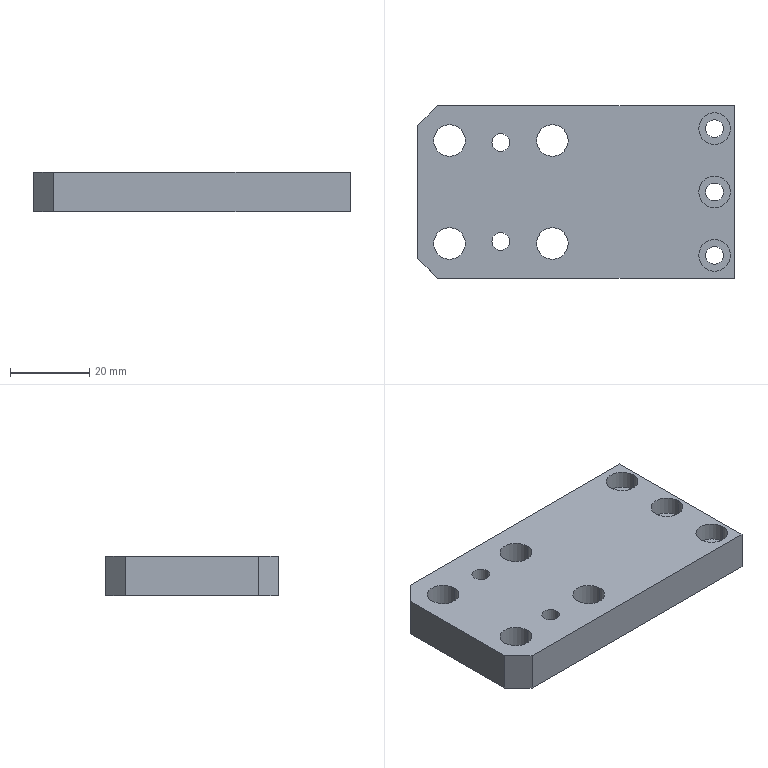Part | SolidWorks | features HoleWzd 3, Chamfer 1, Extrusion 1 | 1 solid | 41 faces | box 80 x 43.6 x 10 mm | volume 31034 mm3 | cylinder 28 | plane 13 | commonest cylinder face diameters 8 x18 4.5 x10
STEP:
#1=CARTESIAN_POINT('',(71.,37.8,-4.6));
#2=VERTEX_POINT('',#1);
#3=CARTESIAN_POINT('',(79.,37.8,-4.6));
#4=VERTEX_POINT('',#3);
#5=CARTESIAN_POINT('',(75.,37.8,-4.6));
#6=DIRECTION('',(0.,0.,1.));
#7=DIRECTION('',(1.,0.,0.));
#8=AXIS2_PLACEMENT_3D('',#5,#6,#7);
#9=CIRCLE('',#8,4.);
#10=EDGE_CURVE('',#2,#4,#9,.T.);
#11=ORIENTED_EDGE('',*,*,#10,.F.);
#12=CARTESIAN_POINT('',(71.,37.8,0.));
#13=VERTEX_POINT('',#12);
#14=CARTESIAN_POINT('',(71.,37.8,0.));
#15=DIRECTION('',(0.,0.,1.));
#16=VECTOR('',#15,1000.);
#17=LINE('',#14,#16);
#18=EDGE_CURVE('',#2,#13,#17,.T.);
#19=ORIENTED_EDGE('',*,*,#18,.T.);
#20=CARTESIAN_POINT('',(79.,37.8,0.));
#21=VERTEX_POINT('',#20);
#22=CARTESIAN_POINT('',(75.,37.8,0.));
#23=DIRECTION('',(0.,0.,1.));
#24=DIRECTION('',(1.,0.,0.));
#25=AXIS2_PLACEMENT_3D('',#22,#23,#24);
#26=CIRCLE('',#25,4.);
#27=EDGE_CURVE('',#13,#21,#26,.T.);
#28=ORIENTED_EDGE('',*,*,#27,.T.);
#29=CARTESIAN_POINT('',(79.,37.8,0.));
#30=DIRECTION('',(0.,0.,1.));
#31=VECTOR('',#30,1000.);
#32=LINE('',#29,#31);
#33=EDGE_CURVE('',#4,#21,#32,.T.);
#34=ORIENTED_EDGE('',*,*,#33,.F.);
#35=EDGE_LOOP('',(#11,#19,#28,#34));
#36=FACE_OUTER_BOUND('',#35,.T.);
#37=CARTESIAN_POINT('',(75.,37.8,0.));
#38=DIRECTION('',(0.,0.,1.));
#39=DIRECTION('',(1.,0.,0.));
#40=AXIS2_PLACEMENT_3D('',#37,#38,#39);
#41=CYLINDRICAL_SURFACE('',#40,4.);
#42=ADVANCED_FACE('',(#36),#41,.F.);
#43=CARTESIAN_POINT('',(72.75,37.8,-10.));
#44=VERTEX_POINT('',#43);
#45=CARTESIAN_POINT('',(77.25,37.8,-10.));
#46=VERTEX_POINT('',#45);
#47=CARTESIAN_POINT('',(75.,37.8,-10.));
#48=DIRECTION('',(0.,0.,1.));
#49=DIRECTION('',(1.,0.,0.));
#50=AXIS2_PLACEMENT_3D('',#47,#48,#49);
#51=CIRCLE('',#50,2.25);
#52=EDGE_CURVE('',#44,#46,#51,.T.);
#53=ORIENTED_EDGE('',*,*,#52,.F.);
#54=CARTESIAN_POINT('',(72.75,37.8,-4.6));
#55=VERTEX_POINT('',#54);
#56=CARTESIAN_POINT('',(72.75,37.8,0.));
#57=DIRECTION('',(0.,0.,1.));
#58=VECTOR('',#57,1000.);
#59=LINE('',#56,#58);
#60=EDGE_CURVE('',#44,#55,#59,.T.);
#61=ORIENTED_EDGE('',*,*,#60,.T.);
#62=CARTESIAN_POINT('',(77.25,37.8,-4.6));
#63=VERTEX_POINT('',#62);
#64=CARTESIAN_POINT('',(75.,37.8,-4.6));
#65=DIRECTION('',(0.,0.,1.));
#66=DIRECTION('',(1.,0.,0.));
#67=AXIS2_PLACEMENT_3D('',#64,#65,#66);
#68=CIRCLE('',#67,2.25);
#69=EDGE_CURVE('',#55,#63,#68,.T.);
#70=ORIENTED_EDGE('',*,*,#69,.T.);
#71=CARTESIAN_POINT('',(77.25,37.8,0.));
#72=DIRECTION('',(0.,0.,1.));
#73=VECTOR('',#72,1000.);
#74=LINE('',#71,#73);
#75=EDGE_CURVE('',#46,#63,#74,.T.);
#76=ORIENTED_EDGE('',*,*,#75,.F.);
#77=EDGE_LOOP('',(#53,#61,#70,#76));
#78=FACE_OUTER_BOUND('',#77,.T.);
#79=CARTESIAN_POINT('',(75.,37.8,0.));
#80=DIRECTION('',(0.,0.,1.));
#81=DIRECTION('',(1.,0.,0.));
#82=AXIS2_PLACEMENT_3D('',#79,#80,#81);
#83=CYLINDRICAL_SURFACE('',#82,2.25);
#84=ADVANCED_FACE('',(#78),#83,.F.);
#85=CARTESIAN_POINT('',(71.,5.8,-4.6));
#86=VERTEX_POINT('',#85);
#87=CARTESIAN_POINT('',(79.,5.8,-4.6));
#88=VERTEX_POINT('',#87);
#89=CARTESIAN_POINT('',(75.,5.8,-4.6));
#90=DIRECTION('',(0.,0.,1.));
#91=DIRECTION('',(1.,0.,0.));
#92=AXIS2_PLACEMENT_3D('',#89,#90,#91);
#93=CIRCLE('',#92,4.);
#94=EDGE_CURVE('',#86,#88,#93,.T.);
#95=ORIENTED_EDGE('',*,*,#94,.F.);
#96=CARTESIAN_POINT('',(71.,5.8,0.));
#97=VERTEX_POINT('',#96);
#98=CARTESIAN_POINT('',(71.,5.8,0.));
#99=DIRECTION('',(0.,0.,1.));
#100=VECTOR('',#99,1000.);
#101=LINE('',#98,#100);
#102=EDGE_CURVE('',#86,#97,#101,.T.);
#103=ORIENTED_EDGE('',*,*,#102,.T.);
#104=CARTESIAN_POINT('',(79.,5.8,0.));
#105=VERTEX_POINT('',#104);
#106=CARTESIAN_POINT('',(75.,5.8,0.));
#107=DIRECTION('',(0.,0.,1.));
#108=DIRECTION('',(1.,0.,0.));
#109=AXIS2_PLACEMENT_3D('',#106,#107,#108);
#110=CIRCLE('',#109,4.);
#111=EDGE_CURVE('',#97,#105,#110,.T.);
#112=ORIENTED_EDGE('',*,*,#111,.T.);
#113=CARTESIAN_POINT('',(79.,5.8,0.));
#114=DIRECTION('',(0.,0.,1.));
#115=VECTOR('',#114,1000.);
#116=LINE('',#113,#115);
#117=EDGE_CURVE('',#88,#105,#116,.T.);
#118=ORIENTED_EDGE('',*,*,#117,.F.);
#119=EDGE_LOOP('',(#95,#103,#112,#118));
#120=FACE_OUTER_BOUND('',#119,.T.);
#121=CARTESIAN_POINT('',(75.,5.8,0.));
#122=DIRECTION('',(0.,0.,1.));
#123=DIRECTION('',(1.,0.,0.));
#124=AXIS2_PLACEMENT_3D('',#121,#122,#123);
#125=CYLINDRICAL_SURFACE('',#124,4.);
#126=ADVANCED_FACE('',(#120),#125,.F.);
#127=CARTESIAN_POINT('',(72.75,5.8,-10.));
#128=VERTEX_POINT('',#127);
#129=CARTESIAN_POINT('',(77.25,5.8,-10.));
#130=VERTEX_POINT('',#129);
#131=CARTESIAN_POINT('',(75.,5.8,-10.));
#132=DIRECTION('',(0.,0.,1.));
#133=DIRECTION('',(1.,0.,0.));
#134=AXIS2_PLACEMENT_3D('',#131,#132,#133);
#135=CIRCLE('',#134,2.25);
#136=EDGE_CURVE('',#128,#130,#135,.T.);
#137=ORIENTED_EDGE('',*,*,#136,.F.);
#138=CARTESIAN_POINT('',(72.75,5.8,-4.6));
#139=VERTEX_POINT('',#138);
#140=CARTESIAN_POINT('',(72.75,5.8,0.));
#141=DIRECTION('',(0.,0.,1.));
#142=VECTOR('',#141,1000.);
#143=LINE('',#140,#142);
#144=EDGE_CURVE('',#128,#139,#143,.T.);
#145=ORIENTED_EDGE('',*,*,#144,.T.);
#146=CARTESIAN_POINT('',(77.25,5.8,-4.6));
#147=VERTEX_POINT('',#146);
#148=CARTESIAN_POINT('',(75.,5.8,-4.6));
#149=DIRECTION('',(0.,0.,1.));
#150=DIRECTION('',(1.,0.,0.));
#151=AXIS2_PLACEMENT_3D('',#148,#149,#150);
#152=CIRCLE('',#151,2.25);
#153=EDGE_CURVE('',#139,#147,#152,.T.);
#154=ORIENTED_EDGE('',*,*,#153,.T.);
#155=CARTESIAN_POINT('',(77.25,5.8,0.));
#156=DIRECTION('',(0.,0.,1.));
#157=VECTOR('',#156,1000.);
#158=LINE('',#155,#157);
#159=EDGE_CURVE('',#130,#147,#158,.T.);
#160=ORIENTED_EDGE('',*,*,#159,.F.);
#161=EDGE_LOOP('',(#137,#145,#154,#160));
#162=FACE_OUTER_BOUND('',#161,.T.);
#163=CARTESIAN_POINT('',(75.,5.8,0.));
#164=DIRECTION('',(0.,0.,1.));
#165=DIRECTION('',(1.,0.,0.));
#166=AXIS2_PLACEMENT_3D('',#163,#164,#165);
#167=CYLINDRICAL_SURFACE('',#166,2.25);
#168=ADVANCED_FACE('',(#162),#167,.F.);
#169=CARTESIAN_POINT('',(71.,21.8,-4.6));
#170=VERTEX_POINT('',#169);
#171=CARTESIAN_POINT('',(79.,21.8,-4.6));
#172=VERTEX_POINT('',#171);
#173=CARTESIAN_POINT('',(75.,21.8,-4.6));
#174=DIRECTION('',(0.,0.,1.));
#175=DIRECTION('',(1.,0.,0.));
#176=AXIS2_PLACEMENT_3D('',#173,#174,#175);
#177=CIRCLE('',#176,4.);
#178=EDGE_CURVE('',#170,#172,#177,.T.);
#179=ORIENTED_EDGE('',*,*,#178,.F.);
#180=CARTESIAN_POINT('',(71.,21.8,0.));
#181=VERTEX_POINT('',#180);
#182=CARTESIAN_POINT('',(71.,21.8,0.));
#183=DIRECTION('',(0.,0.,1.));
#184=VECTOR('',#183,1000.);
#185=LINE('',#182,#184);
#186=EDGE_CURVE('',#170,#181,#185,.T.);
#187=ORIENTED_EDGE('',*,*,#186,.T.);
#188=CARTESIAN_POINT('',(79.,21.8,0.));
#189=VERTEX_POINT('',#188);
#190=CARTESIAN_POINT('',(75.,21.8,0.));
#191=DIRECTION('',(0.,0.,1.));
#192=DIRECTION('',(1.,0.,0.));
#193=AXIS2_PLACEMENT_3D('',#190,#191,#192);
#194=CIRCLE('',#193,4.);
#195=EDGE_CURVE('',#181,#189,#194,.T.);
#196=ORIENTED_EDGE('',*,*,#195,.T.);
#197=CARTESIAN_POINT('',(79.,21.8,0.));
#198=DIRECTION('',(0.,0.,1.));
#199=VECTOR('',#198,1000.);
#200=LINE('',#197,#199);
#201=EDGE_CURVE('',#172,#189,#200,.T.);
#202=ORIENTED_EDGE('',*,*,#201,.F.);
#203=EDGE_LOOP('',(#179,#187,#196,#202));
#204=FACE_OUTER_BOUND('',#203,.T.);
#205=CARTESIAN_POINT('',(75.,21.8,0.));
#206=DIRECTION('',(0.,0.,1.));
#207=DIRECTION('',(1.,0.,0.));
#208=AXIS2_PLACEMENT_3D('',#205,#206,#207);
#209=CYLINDRICAL_SURFACE('',#208,4.);
#210=ADVANCED_FACE('',(#204),#209,.F.);
#211=CARTESIAN_POINT('',(72.75,21.8,-10.));
#212=VERTEX_POINT('',#211);
#213=CARTESIAN_POINT('',(77.25,21.8,-10.));
#214=VERTEX_POINT('',#213);
#215=CARTESIAN_POINT('',(75.,21.8,-10.));
#216=DIRECTION('',(0.,0.,1.));
#217=DIRECTION('',(1.,0.,0.));
#218=AXIS2_PLACEMENT_3D('',#215,#216,#217);
#219=CIRCLE('',#218,2.25);
#220=EDGE_CURVE('',#212,#214,#219,.T.);
#221=ORIENTED_EDGE('',*,*,#220,.F.);
#222=CARTESIAN_POINT('',(72.75,21.8,-4.6));
#223=VERTEX_POINT('',#222);
#224=CARTESIAN_POINT('',(72.75,21.8,0.));
#225=DIRECTION('',(0.,0.,1.));
#226=VECTOR('',#225,1000.);
#227=LINE('',#224,#226);
#228=EDGE_CURVE('',#212,#223,#227,.T.);
#229=ORIENTED_EDGE('',*,*,#228,.T.);
#230=CARTESIAN_POINT('',(77.25,21.8,-4.6));
#231=VERTEX_POINT('',#230);
#232=CARTESIAN_POINT('',(75.,21.8,-4.6));
#233=DIRECTION('',(0.,0.,1.));
#234=DIRECTION('',(1.,0.,0.));
#235=AXIS2_PLACEMENT_3D('',#232,#233,#234);
#236=CIRCLE('',#235,2.25);
#237=EDGE_CURVE('',#223,#231,#236,.T.);
#238=ORIENTED_EDGE('',*,*,#237,.T.);
#239=CARTESIAN_POINT('',(77.25,21.8,0.));
#240=DIRECTION('',(0.,0.,1.));
#241=VECTOR('',#240,1000.);
#242=LINE('',#239,#241);
#243=EDGE_CURVE('',#214,#231,#242,.T.);
#244=ORIENTED_EDGE('',*,*,#243,.F.);
#245=EDGE_LOOP('',(#221,#229,#238,#244));
#246=FACE_OUTER_BOUND('',#245,.T.);
#247=CARTESIAN_POINT('',(75.,21.8,0.));
#248=DIRECTION('',(0.,0.,1.));
#249=DIRECTION('',(1.,0.,0.));
#250=AXIS2_PLACEMENT_3D('',#247,#248,#249);
#251=CYLINDRICAL_SURFACE('',#250,2.25);
#252=ADVANCED_FACE('',(#246),#251,.F.);
#253=CARTESIAN_POINT('',(25.,34.3,-5.4));
#254=VERTEX_POINT('',#253);
#255=CARTESIAN_POINT('',(17.,34.3,-5.4));
#256=VERTEX_POINT('',#255);
#257=CARTESIAN_POINT('',(21.,34.3,-5.4));
#258=DIRECTION('',(0.,0.,-1.));
#259=DIRECTION('',(-1.,0.,0.));
#260=AXIS2_PLACEMENT_3D('',#257,#258,#259);
#261=CIRCLE('',#260,4.);
#262=EDGE_CURVE('',#254,#256,#261,.T.);
#263=ORIENTED_EDGE('',*,*,#262,.F.);
#264=CARTESIAN_POINT('',(25.,34.3,-10.));
#265=VERTEX_POINT('',#264);
#266=CARTESIAN_POINT('',(25.,34.3,-10.));
#267=DIRECTION('',(0.,0.,-1.));
#268=VECTOR('',#267,1000.);
#269=LINE('',#266,#268);
#270=EDGE_CURVE('',#254,#265,#269,.T.);
#271=ORIENTED_EDGE('',*,*,#270,.T.);
#272=CARTESIAN_POINT('',(17.,34.3,-10.));
#273=VERTEX_POINT('',#272);
#274=CARTESIAN_POINT('',(21.,34.3,-10.));
#275=DIRECTION('',(0.,0.,-1.));
#276=DIRECTION('',(-1.,0.,0.));
#277=AXIS2_PLACEMENT_3D('',#274,#275,#276);
#278=CIRCLE('',#277,4.);
#279=EDGE_CURVE('',#265,#273,#278,.T.);
#280=ORIENTED_EDGE('',*,*,#279,.T.);
#281=CARTESIAN_POINT('',(17.,34.3,-10.));
#282=DIRECTION('',(0.,0.,-1.));
#283=VECTOR('',#282,1000.);
#284=LINE('',#281,#283);
#285=EDGE_CURVE('',#256,#273,#284,.T.);
#286=ORIENTED_EDGE('',*,*,#285,.F.);
#287=EDGE_LOOP('',(#263,#271,#280,#286));
#288=FACE_OUTER_BOUND('',#287,.T.);
#289=CARTESIAN_POINT('',(21.,34.3,-10.));
#290=DIRECTION('',(0.,0.,-1.));
#291=DIRECTION('',(-1.,0.,0.));
#292=AXIS2_PLACEMENT_3D('',#289,#290,#291);
#293=CYLINDRICAL_SURFACE('',#292,4.);
#294=ADVANCED_FACE('',(#288),#293,.F.);
#295=CARTESIAN_POINT('',(23.25,34.3,0.));
#296=VERTEX_POINT('',#295);
#297=CARTESIAN_POINT('',(18.75,34.3,0.));
#298=VERTEX_POINT('',#297);
#299=CARTESIAN_POINT('',(21.,34.3,0.));
#300=DIRECTION('',(0.,0.,-1.));
#301=DIRECTION('',(-1.,0.,0.));
#302=AXIS2_PLACEMENT_3D('',#299,#300,#301);
#303=CIRCLE('',#302,2.25);
#304=EDGE_CURVE('',#296,#298,#303,.T.);
#305=ORIENTED_EDGE('',*,*,#304,.F.);
#306=CARTESIAN_POINT('',(23.25,34.3,-5.4));
#307=VERTEX_POINT('',#306);
#308=CARTESIAN_POINT('',(23.25,34.3,-10.));
#309=DIRECTION('',(0.,0.,-1.));
#310=VECTOR('',#309,1000.);
#311=LINE('',#308,#310);
#312=EDGE_CURVE('',#296,#307,#311,.T.);
#313=ORIENTED_EDGE('',*,*,#312,.T.);
#314=CARTESIAN_POINT('',(18.75,34.3,-5.4));
#315=VERTEX_POINT('',#314);
#316=CARTESIAN_POINT('',(21.,34.3,-5.4));
#317=DIRECTION('',(0.,0.,-1.));
#318=DIRECTION('',(-1.,0.,0.));
#319=AXIS2_PLACEMENT_3D('',#316,#317,#318);
#320=CIRCLE('',#319,2.25);
#321=EDGE_CURVE('',#307,#315,#320,.T.);
#322=ORIENTED_EDGE('',*,*,#321,.T.);
#323=CARTESIAN_POINT('',(18.75,34.3,-10.));
#324=DIRECTION('',(0.,0.,-1.));
#325=VECTOR('',#324,1000.);
#326=LINE('',#323,#325);
#327=EDGE_CURVE('',#298,#315,#326,.T.);
#328=ORIENTED_EDGE('',*,*,#327,.F.);
#329=EDGE_LOOP('',(#305,#313,#322,#328));
#330=FACE_OUTER_BOUND('',#329,.T.);
#331=CARTESIAN_POINT('',(21.,34.3,-10.));
#332=DIRECTION('',(0.,0.,-1.));
#333=DIRECTION('',(-1.,0.,0.));
#334=AXIS2_PLACEMENT_3D('',#331,#332,#333);
#335=CYLINDRICAL_SURFACE('',#334,2.25);
#336=ADVANCED_FACE('',(#330),#335,.F.);
#337=CARTESIAN_POINT('',(25.,9.3,-5.4));
#338=VERTEX_POINT('',#337);
#339=CARTESIAN_POINT('',(17.,9.3,-5.4));
#340=VERTEX_POINT('',#339);
#341=CARTESIAN_POINT('',(21.,9.3,-5.4));
#342=DIRECTION('',(0.,0.,-1.));
#343=DIRECTION('',(-1.,0.,0.));
#344=AXIS2_PLACEMENT_3D('',#341,#342,#343);
#345=CIRCLE('',#344,4.);
#346=EDGE_CURVE('',#338,#340,#345,.T.);
#347=ORIENTED_EDGE('',*,*,#346,.F.);
#348=CARTESIAN_POINT('',(25.,9.3,-10.));
#349=VERTEX_POINT('',#348);
#350=CARTESIAN_POINT('',(25.,9.3,-10.));
#351=DIRECTION('',(0.,0.,-1.));
#352=VECTOR('',#351,1000.);
#353=LINE('',#350,#352);
#354=EDGE_CURVE('',#338,#349,#353,.T.);
#355=ORIENTED_EDGE('',*,*,#354,.T.);
#356=CARTESIAN_POINT('',(17.,9.3,-10.));
#357=VERTEX_POINT('',#356);
#358=CARTESIAN_POINT('',(21.,9.3,-10.));
#359=DIRECTION('',(0.,0.,-1.));
#360=DIRECTION('',(-1.,0.,0.));
#361=AXIS2_PLACEMENT_3D('',#358,#359,#360);
#362=CIRCLE('',#361,4.);
#363=EDGE_CURVE('',#349,#357,#362,.T.);
#364=ORIENTED_EDGE('',*,*,#363,.T.);
#365=CARTESIAN_POINT('',(17.,9.3,-10.));
#366=DIRECTION('',(0.,0.,-1.));
#367=VECTOR('',#366,1000.);
#368=LINE('',#365,#367);
#369=EDGE_CURVE('',#340,#357,#368,.T.);
#370=ORIENTED_EDGE('',*,*,#369,.F.);
#371=EDGE_LOOP('',(#347,#355,#364,#370));
#372=FACE_OUTER_BOUND('',#371,.T.);
#373=CARTESIAN_POINT('',(21.,9.3,-10.));
#374=DIRECTION('',(0.,0.,-1.));
#375=DIRECTION('',(-1.,0.,0.));
#376=AXIS2_PLACEMENT_3D('',#373,#374,#375);
#377=CYLINDRICAL_SURFACE('',#376,4.);
#378=ADVANCED_FACE('',(#372),#377,.F.);
#379=CARTESIAN_POINT('',(23.25,9.3,0.));
#380=VERTEX_POINT('',#379);
#381=CARTESIAN_POINT('',(18.75,9.3,0.));
#382=VERTEX_POINT('',#381);
#383=CARTESIAN_POINT('',(21.,9.3,0.));
#384=DIRECTION('',(0.,0.,-1.));
#385=DIRECTION('',(-1.,0.,0.));
#386=AXIS2_PLACEMENT_3D('',#383,#384,#385);
#387=CIRCLE('',#386,2.25);
#388=EDGE_CURVE('',#380,#382,#387,.T.);
#389=ORIENTED_EDGE('',*,*,#388,.F.);
#390=CARTESIAN_POINT('',(23.25,9.3,-5.4));
#391=VERTEX_POINT('',#390);
#392=CARTESIAN_POINT('',(23.25,9.3,-10.));
#393=DIRECTION('',(0.,0.,-1.));
#394=VECTOR('',#393,1000.);
#395=LINE('',#392,#394);
#396=EDGE_CURVE('',#380,#391,#395,.T.);
#397=ORIENTED_EDGE('',*,*,#396,.T.);
#398=CARTESIAN_POINT('',(18.75,9.3,-5.4));
#399=VERTEX_POINT('',#398);
#400=CARTESIAN_POINT('',(21.,9.3,-5.4));
#401=DIRECTION('',(0.,0.,-1.));
#402=DIRECTION('',(-1.,0.,0.));
#403=AXIS2_PLACEMENT_3D('',#400,#401,#402);
#404=CIRCLE('',#403,2.25);
#405=EDGE_CURVE('',#391,#399,#404,.T.);
#406=ORIENTED_EDGE('',*,*,#405,.T.);
#407=CARTESIAN_POINT('',(18.75,9.3,-10.));
#408=DIRECTION('',(0.,0.,-1.));
#409=VECTOR('',#408,1000.);
#410=LINE('',#407,#409);
#411=EDGE_CURVE('',#382,#399,#410,.T.);
#412=ORIENTED_EDGE('',*,*,#411,.F.);
#413=EDGE_LOOP('',(#389,#397,#406,#412));
#414=FACE_OUTER_BOUND('',#413,.T.);
#415=CARTESIAN_POINT('',(21.,9.3,-10.));
#416=DIRECTION('',(0.,0.,-1.));
#417=DIRECTION('',(-1.,0.,0.));
#418=AXIS2_PLACEMENT_3D('',#415,#416,#417);
#419=CYLINDRICAL_SURFACE('',#418,2.25);
#420=ADVANCED_FACE('',(#414),#419,.F.);
#421=CARTESIAN_POINT('',(38.043,34.8,0.));
#422=VERTEX_POINT('',#421);
#423=CARTESIAN_POINT('',(30.043,34.8,0.));
#424=VERTEX_POINT('',#423);
#425=CARTESIAN_POINT('',(34.043,34.8,0.));
#426=DIRECTION('',(0.,0.,-1.));
#427=DIRECTION('',(-1.,0.,0.));
#428=AXIS2_PLACEMENT_3D('',#425,#426,#427);
#429=CIRCLE('',#428,4.);
#430=EDGE_CURVE('',#422,#424,#429,.T.);
#431=ORIENTED_EDGE('',*,*,#430,.F.);
#432=CARTESIAN_POINT('',(38.043,34.8,-10.));
#433=VERTEX_POINT('',#432);
#434=CARTESIAN_POINT('',(38.043,34.8,-10.));
#435=DIRECTION('',(0.,0.,-1.));
#436=VECTOR('',#435,1000.);
#437=LINE('',#434,#436);
#438=EDGE_CURVE('',#422,#433,#437,.T.);
#439=ORIENTED_EDGE('',*,*,#438,.T.);
#440=CARTESIAN_POINT('',(30.043,34.8,-10.));
#441=VERTEX_POINT('',#440);
#442=CARTESIAN_POINT('',(34.043,34.8,-10.));
#443=DIRECTION('',(0.,0.,-1.));
#444=DIRECTION('',(-1.,0.,0.));
#445=AXIS2_PLACEMENT_3D('',#442,#443,#444);
#446=CIRCLE('',#445,4.);
#447=EDGE_CURVE('',#433,#441,#446,.T.);
#448=ORIENTED_EDGE('',*,*,#447,.T.);
#449=CARTESIAN_POINT('',(30.043,34.8,-10.));
#450=DIRECTION('',(0.,0.,-1.));
#451=VECTOR('',#450,1000.);
#452=LINE('',#449,#451);
#453=EDGE_CURVE('',#424,#441,#452,.T.);
#454=ORIENTED_EDGE('',*,*,#453,.F.);
#455=EDGE_LOOP('',(#431,#439,#448,#454));
#456=FACE_OUTER_BOUND('',#455,.T.);
#457=CARTESIAN_POINT('',(34.043,34.8,-10.));
#458=DIRECTION('',(0.,0.,-1.));
#459=DIRECTION('',(-1.,0.,0.));
#460=AXIS2_PLACEMENT_3D('',#457,#458,#459);
#461=CYLINDRICAL_SURFACE('',#460,4.);
#462=ADVANCED_FACE('',(#456),#461,.F.);
#463=CARTESIAN_POINT('',(12.043,34.8,0.));
#464=VERTEX_POINT('',#463);
#465=CARTESIAN_POINT('',(4.043,34.8,0.));
#466=VERTEX_POINT('',#465);
#467=CARTESIAN_POINT('',(8.043,34.8,0.));
#468=DIRECTION('',(0.,0.,-1.));
#469=DIRECTION('',(-1.,0.,0.));
#470=AXIS2_PLACEMENT_3D('',#467,#468,#469);
#471=CIRCLE('',#470,4.);
#472=EDGE_CURVE('',#464,#466,#471,.T.);
#473=ORIENTED_EDGE('',*,*,#472,.F.);
#474=CARTESIAN_POINT('',(12.043,34.8,-10.));
#475=VERTEX_POINT('',#474);
#476=CARTESIAN_POINT('',(12.043,34.8,-10.));
#477=DIRECTION('',(0.,0.,-1.));
#478=VECTOR('',#477,1000.);
#479=LINE('',#476,#478);
#480=EDGE_CURVE('',#464,#475,#479,.T.);
#481=ORIENTED_EDGE('',*,*,#480,.T.);
#482=CARTESIAN_POINT('',(4.043,34.8,-10.));
#483=VERTEX_POINT('',#482);
#484=CARTESIAN_POINT('',(8.043,34.8,-10.));
#485=DIRECTION('',(0.,0.,-1.));
#486=DIRECTION('',(-1.,0.,0.));
#487=AXIS2_PLACEMENT_3D('',#484,#485,#486);
#488=CIRCLE('',#487,4.);
#489=EDGE_CURVE('',#475,#483,#488,.T.);
#490=ORIENTED_EDGE('',*,*,#489,.T.);
#491=CARTESIAN_POINT('',(4.043,34.8,-10.));
#492=DIRECTION('',(0.,0.,-1.));
#493=VECTOR('',#492,1000.);
#494=LINE('',#491,#493);
#495=EDGE_CURVE('',#466,#483,#494,.T.);
#496=ORIENTED_EDGE('',*,*,#495,.F.);
#497=EDGE_LOOP('',(#473,#481,#490,#496));
#498=FACE_OUTER_BOUND('',#497,.T.);
#499=CARTESIAN_POINT('',(8.043,34.8,-10.));
#500=DIRECTION('',(0.,0.,-1.));
#501=DIRECTION('',(-1.,0.,0.));
#502=AXIS2_PLACEMENT_3D('',#499,#500,#501);
#503=CYLINDRICAL_SURFACE('',#502,4.);
#504=ADVANCED_FACE('',(#498),#503,.F.);
#505=CARTESIAN_POINT('',(12.043,8.8,0.));
#506=VERTEX_POINT('',#505);
#507=CARTESIAN_POINT('',(4.043,8.8,0.));
#508=VERTEX_POINT('',#507);
#509=CARTESIAN_POINT('',(8.043,8.8,0.));
#510=DIRECTION('',(0.,0.,-1.));
#511=DIRECTION('',(-1.,0.,0.));
#512=AXIS2_PLACEMENT_3D('',#509,#510,#511);
#513=CIRCLE('',#512,4.);
#514=EDGE_CURVE('',#506,#508,#513,.T.);
#515=ORIENTED_EDGE('',*,*,#514,.F.);
#516=CARTESIAN_POINT('',(12.043,8.8,-10.));
#517=VERTEX_POINT('',#516);
#518=CARTESIAN_POINT('',(12.043,8.8,-10.));
#519=DIRECTION('',(0.,0.,-1.));
#520=VECTOR('',#519,1000.);
#521=LINE('',#518,#520);
#522=EDGE_CURVE('',#506,#517,#521,.T.);
#523=ORIENTED_EDGE('',*,*,#522,.T.);
#524=CARTESIAN_POINT('',(4.043,8.8,-10.));
#525=VERTEX_POINT('',#524);
#526=CARTESIAN_POINT('',(8.043,8.8,-10.));
#527=DIRECTION('',(0.,0.,-1.));
#528=DIRECTION('',(-1.,0.,0.));
#529=AXIS2_PLACEMENT_3D('',#526,#527,#528);
#530=CIRCLE('',#529,4.);
#531=EDGE_CURVE('',#517,#525,#530,.T.);
#532=ORIENTED_EDGE('',*,*,#531,.T.);
#533=CARTESIAN_POINT('',(4.043,8.8,-10.));
#534=DIRECTION('',(0.,0.,-1.));
#535=VECTOR('',#534,1000.);
#536=LINE('',#533,#535);
#537=EDGE_CURVE('',#508,#525,#536,.T.);
#538=ORIENTED_EDGE('',*,*,#537,.F.);
#539=EDGE_LOOP('',(#515,#523,#532,#538));
#540=FACE_OUTER_BOUND('',#539,.T.);
#541=CARTESIAN_POINT('',(8.043,8.8,-10.));
#542=DIRECTION('',(0.,0.,-1.));
#543=DIRECTION('',(-1.,0.,0.));
#544=AXIS2_PLACEMENT_3D('',#541,#542,#543);
#545=CYLINDRICAL_SURFACE('',#544,4.);
#546=ADVANCED_FACE('',(#540),#545,.F.);
#547=CARTESIAN_POINT('',(38.043,8.8,0.));
#548=VERTEX_POINT('',#547);
#549=CARTESIAN_POINT('',(30.043,8.8,0.));
#550=VERTEX_POINT('',#549);
#551=CARTESIAN_POINT('',(34.043,8.8,0.));
#552=DIRECTION('',(0.,0.,-1.));
#553=DIRECTION('',(-1.,0.,0.));
#554=AXIS2_PLACEMENT_3D('',#551,#552,#553);
#555=CIRCLE('',#554,4.);
#556=EDGE_CURVE('',#548,#550,#555,.T.);
#557=ORIENTED_EDGE('',*,*,#556,.F.);
#558=CARTESIAN_POINT('',(38.043,8.8,-10.));
#559=VERTEX_POINT('',#558);
#560=CARTESIAN_POINT('',(38.043,8.8,-10.));
#561=DIRECTION('',(0.,0.,-1.));
#562=VECTOR('',#561,1000.);
#563=LINE('',#560,#562);
#564=EDGE_CURVE('',#548,#559,#563,.T.);
#565=ORIENTED_EDGE('',*,*,#564,.T.);
#566=CARTESIAN_POINT('',(30.043,8.8,-10.));
#567=VERTEX_POINT('',#566);
#568=CARTESIAN_POINT('',(34.043,8.8,-10.));
#569=DIRECTION('',(0.,0.,-1.));
#570=DIRECTION('',(-1.,0.,0.));
#571=AXIS2_PLACEMENT_3D('',#568,#569,#570);
#572=CIRCLE('',#571,4.);
#573=EDGE_CURVE('',#559,#567,#572,.T.);
#574=ORIENTED_EDGE('',*,*,#573,.T.);
#575=CARTESIAN_POINT('',(30.043,8.8,-10.));
#576=DIRECTION('',(0.,0.,-1.));
#577=VECTOR('',#576,1000.);
#578=LINE('',#575,#577);
#579=EDGE_CURVE('',#550,#567,#578,.T.);
#580=ORIENTED_EDGE('',*,*,#579,.F.);
#581=EDGE_LOOP('',(#557,#565,#574,#580));
#582=FACE_OUTER_BOUND('',#581,.T.);
#583=CARTESIAN_POINT('',(34.043,8.8,-10.));
#584=DIRECTION('',(0.,0.,-1.));
#585=DIRECTION('',(-1.,0.,0.));
#586=AXIS2_PLACEMENT_3D('',#583,#584,#585);
#587=CYLINDRICAL_SURFACE('',#586,4.);
#588=ADVANCED_FACE('',(#582),#587,.F.);
#589=CARTESIAN_POINT('',(0.,38.6,-10.));
#590=VERTEX_POINT('',#589);
#591=CARTESIAN_POINT('',(0.,5.,-10.));
#592=VERTEX_POINT('',#591);
#593=CARTESIAN_POINT('',(0.,43.6,-10.));
#594=DIRECTION('',(0.,-1.,0.));
#595=VECTOR('',#594,1000.);
#596=LINE('',#593,#595);
#597=EDGE_CURVE('',#590,#592,#596,.T.);
#598=ORIENTED_EDGE('',*,*,#597,.T.);
#599=CARTESIAN_POINT('',(0.,5.,0.));
#600=VERTEX_POINT('',#599);
#601=CARTESIAN_POINT('',(0.,5.,0.));
#602=DIRECTION('',(0.,0.,1.));
#603=VECTOR('',#602,1000.);
#604=LINE('',#601,#603);
#605=EDGE_CURVE('',#592,#600,#604,.T.);
#606=ORIENTED_EDGE('',*,*,#605,.T.);
#607=CARTESIAN_POINT('',(0.,38.6,0.));
#608=VERTEX_POINT('',#607);
#609=CARTESIAN_POINT('',(0.,43.6,0.));
#610=DIRECTION('',(0.,-1.,0.));
#611=VECTOR('',#610,1000.);
#612=LINE('',#609,#611);
#613=EDGE_CURVE('',#608,#600,#612,.T.);
#614=ORIENTED_EDGE('',*,*,#613,.F.);
#615=CARTESIAN_POINT('',(0.,38.6,0.));
#616=DIRECTION('',(0.,0.,-1.));
#617=VECTOR('',#616,1000.);
#618=LINE('',#615,#617);
#619=EDGE_CURVE('',#608,#590,#618,.T.);
#620=ORIENTED_EDGE('',*,*,#619,.T.);
#621=EDGE_LOOP('',(#598,#606,#614,#620));
#622=FACE_OUTER_BOUND('',#621,.T.);
#623=CARTESIAN_POINT('',(0.,43.6,0.));
#624=DIRECTION('',(1.,0.,0.));
#625=DIRECTION('',(0.,0.,-1.));
#626=AXIS2_PLACEMENT_3D('',#623,#624,#625);
#627=PLANE('',#626);
#628=ADVANCED_FACE('',(#622),#627,.F.);
#629=CARTESIAN_POINT('',(75.,37.8,0.));
#630=DIRECTION('',(0.,0.,1.));
#631=DIRECTION('',(1.,0.,0.));
#632=AXIS2_PLACEMENT_3D('',#629,#630,#631);
#633=CIRCLE('',#632,4.);
#634=EDGE_CURVE('',#21,#13,#633,.T.);
#635=ORIENTED_EDGE('',*,*,#634,.F.);
#636=ORIENTED_EDGE('',*,*,#27,.F.);
#637=EDGE_LOOP('',(#635,#636));
#638=FACE_BOUND('',#637,.T.);
#639=CARTESIAN_POINT('',(75.,5.8,0.));
#640=DIRECTION('',(0.,0.,1.));
#641=DIRECTION('',(1.,0.,0.));
#642=AXIS2_PLACEMENT_3D('',#639,#640,#641);
#643=CIRCLE('',#642,4.);
#644=EDGE_CURVE('',#105,#97,#643,.T.);
#645=ORIENTED_EDGE('',*,*,#644,.F.);
#646=ORIENTED_EDGE('',*,*,#111,.F.);
#647=EDGE_LOOP('',(#645,#646));
#648=FACE_BOUND('',#647,.T.);
#649=CARTESIAN_POINT('',(75.,21.8,0.));
#650=DIRECTION('',(0.,0.,1.));
#651=DIRECTION('',(1.,0.,0.));
#652=AXIS2_PLACEMENT_3D('',#649,#650,#651);
#653=CIRCLE('',#652,4.);
#654=EDGE_CURVE('',#189,#181,#653,.T.);
#655=ORIENTED_EDGE('',*,*,#654,.F.);
#656=ORIENTED_EDGE('',*,*,#195,.F.);
#657=EDGE_LOOP('',(#655,#656));
#658=FACE_BOUND('',#657,.T.);
#659=CARTESIAN_POINT('',(21.,34.3,0.));
#660=DIRECTION('',(0.,0.,-1.));
#661=DIRECTION('',(-1.,0.,0.));
#662=AXIS2_PLACEMENT_3D('',#659,#660,#661);
#663=CIRCLE('',#662,2.25);
#664=EDGE_CURVE('',#298,#296,#663,.T.);
#665=ORIENTED_EDGE('',*,*,#664,.T.);
#666=ORIENTED_EDGE('',*,*,#304,.T.);
#667=EDGE_LOOP('',(#665,#666));
#668=FACE_BOUND('',#667,.T.);
#669=CARTESIAN_POINT('',(21.,9.3,0.));
#670=DIRECTION('',(0.,0.,-1.));
#671=DIRECTION('',(-1.,0.,0.));
#672=AXIS2_PLACEMENT_3D('',#669,#670,#671);
#673=CIRCLE('',#672,2.25);
#674=EDGE_CURVE('',#382,#380,#673,.T.);
#675=ORIENTED_EDGE('',*,*,#674,.T.);
#676=ORIENTED_EDGE('',*,*,#388,.T.);
#677=EDGE_LOOP('',(#675,#676));
#678=FACE_BOUND('',#677,.T.);
#679=CARTESIAN_POINT('',(34.043,34.8,0.));
#680=DIRECTION('',(0.,0.,-1.));
#681=DIRECTION('',(-1.,0.,0.));
#682=AXIS2_PLACEMENT_3D('',#679,#680,#681);
#683=CIRCLE('',#682,4.);
#684=EDGE_CURVE('',#424,#422,#683,.T.);
#685=ORIENTED_EDGE('',*,*,#684,.T.);
#686=ORIENTED_EDGE('',*,*,#430,.T.);
#687=EDGE_LOOP('',(#685,#686));
#688=FACE_BOUND('',#687,.T.);
#689=CARTESIAN_POINT('',(8.043,34.8,0.));
#690=DIRECTION('',(0.,0.,-1.));
#691=DIRECTION('',(-1.,0.,0.));
#692=AXIS2_PLACEMENT_3D('',#689,#690,#691);
#693=CIRCLE('',#692,4.);
#694=EDGE_CURVE('',#466,#464,#693,.T.);
#695=ORIENTED_EDGE('',*,*,#694,.T.);
#696=ORIENTED_EDGE('',*,*,#472,.T.);
#697=EDGE_LOOP('',(#695,#696));
#698=FACE_BOUND('',#697,.T.);
#699=CARTESIAN_POINT('',(8.043,8.8,0.));
#700=DIRECTION('',(0.,0.,-1.));
#701=DIRECTION('',(-1.,0.,0.));
#702=AXIS2_PLACEMENT_3D('',#699,#700,#701);
#703=CIRCLE('',#702,4.);
#704=EDGE_CURVE('',#508,#506,#703,.T.);
#705=ORIENTED_EDGE('',*,*,#704,.T.);
#706=ORIENTED_EDGE('',*,*,#514,.T.);
#707=EDGE_LOOP('',(#705,#706));
#708=FACE_BOUND('',#707,.T.);
#709=CARTESIAN_POINT('',(34.043,8.8,0.));
#710=DIRECTION('',(0.,0.,-1.));
#711=DIRECTION('',(-1.,0.,0.));
#712=AXIS2_PLACEMENT_3D('',#709,#710,#711);
#713=CIRCLE('',#712,4.);
#714=EDGE_CURVE('',#550,#548,#713,.T.);
#715=ORIENTED_EDGE('',*,*,#714,.T.);
#716=ORIENTED_EDGE('',*,*,#556,.T.);
#717=EDGE_LOOP('',(#715,#716));
#718=FACE_BOUND('',#717,.T.);
#719=ORIENTED_EDGE('',*,*,#613,.T.);
#720=CARTESIAN_POINT('',(5.,0.,0.));
#721=VERTEX_POINT('',#720);
#722=CARTESIAN_POINT('',(0.,5.,0.));
#723=DIRECTION('',(0.7071,-0.7071,0.));
#724=VECTOR('',#723,1000.);
#725=LINE('',#722,#724);
#726=EDGE_CURVE('',#600,#721,#725,.T.);
#727=ORIENTED_EDGE('',*,*,#726,.T.);
#728=CARTESIAN_POINT('',(80.,0.,0.));
#729=VERTEX_POINT('',#728);
#730=CARTESIAN_POINT('',(0.,0.,0.));
#731=DIRECTION('',(1.,0.,0.));
#732=VECTOR('',#731,1000.);
#733=LINE('',#730,#732);
#734=EDGE_CURVE('',#721,#729,#733,.T.);
#735=ORIENTED_EDGE('',*,*,#734,.T.);
#736=CARTESIAN_POINT('',(80.,43.6,0.));
#737=VERTEX_POINT('',#736);
#738=CARTESIAN_POINT('',(80.,43.6,0.));
#739=DIRECTION('',(0.,-1.,0.));
#740=VECTOR('',#739,1000.);
#741=LINE('',#738,#740);
#742=EDGE_CURVE('',#737,#729,#741,.T.);
#743=ORIENTED_EDGE('',*,*,#742,.F.);
#744=CARTESIAN_POINT('',(5.,43.6,0.));
#745=VERTEX_POINT('',#744);
#746=CARTESIAN_POINT('',(0.,43.6,0.));
#747=DIRECTION('',(1.,0.,0.));
#748=VECTOR('',#747,1000.);
#749=LINE('',#746,#748);
#750=EDGE_CURVE('',#745,#737,#749,.T.);
#751=ORIENTED_EDGE('',*,*,#750,.F.);
#752=CARTESIAN_POINT('',(5.,43.6,0.));
#753=DIRECTION('',(-0.7071,-0.7071,0.));
#754=VECTOR('',#753,1000.);
#755=LINE('',#752,#754);
#756=EDGE_CURVE('',#745,#608,#755,.T.);
#757=ORIENTED_EDGE('',*,*,#756,.T.);
#758=EDGE_LOOP('',(#719,#727,#735,#743,#751,#757));
#759=FACE_OUTER_BOUND('',#758,.T.);
#760=CARTESIAN_POINT('',(0.,43.6,0.));
#761=DIRECTION('',(0.,0.,-1.));
#762=DIRECTION('',(-1.,0.,0.));
#763=AXIS2_PLACEMENT_3D('',#760,#761,#762);
#764=PLANE('',#763);
#765=ADVANCED_FACE('',(#638,#648,#658,#668,#678,#688,#698,#708,#718,#759),#764,.F.);
#766=CARTESIAN_POINT('',(80.,0.,-10.));
#767=VERTEX_POINT('',#766);
#768=CARTESIAN_POINT('',(80.,0.,0.));
#769=DIRECTION('',(0.,0.,-1.));
#770=VECTOR('',#769,1000.);
#771=LINE('',#768,#770);
#772=EDGE_CURVE('',#729,#767,#771,.T.);
#773=ORIENTED_EDGE('',*,*,#772,.T.);
#774=CARTESIAN_POINT('',(80.,43.6,-10.));
#775=VERTEX_POINT('',#774);
#776=CARTESIAN_POINT('',(80.,43.6,-10.));
#777=DIRECTION('',(0.,-1.,0.));
#778=VECTOR('',#777,1000.);
#779=LINE('',#776,#778);
#780=EDGE_CURVE('',#775,#767,#779,.T.);
#781=ORIENTED_EDGE('',*,*,#780,.F.);
#782=CARTESIAN_POINT('',(80.,43.6,0.));
#783=DIRECTION('',(0.,0.,-1.));
#784=VECTOR('',#783,1000.);
#785=LINE('',#782,#784);
#786=EDGE_CURVE('',#737,#775,#785,.T.);
#787=ORIENTED_EDGE('',*,*,#786,.F.);
#788=ORIENTED_EDGE('',*,*,#742,.T.);
#789=EDGE_LOOP('',(#773,#781,#787,#788));
#790=FACE_OUTER_BOUND('',#789,.T.);
#791=CARTESIAN_POINT('',(80.,43.6,0.));
#792=DIRECTION('',(-1.,0.,0.));
#793=DIRECTION('',(0.,0.,1.));
#794=AXIS2_PLACEMENT_3D('',#791,#792,#793);
#795=PLANE('',#794);
#796=ADVANCED_FACE('',(#790),#795,.F.);
#797=CARTESIAN_POINT('',(75.,37.8,-10.));
#798=DIRECTION('',(0.,0.,1.));
#799=DIRECTION('',(1.,0.,0.));
#800=AXIS2_PLACEMENT_3D('',#797,#798,#799);
#801=CIRCLE('',#800,2.25);
#802=EDGE_CURVE('',#46,#44,#801,.T.);
#803=ORIENTED_EDGE('',*,*,#802,.T.);
#804=ORIENTED_EDGE('',*,*,#52,.T.);
#805=EDGE_LOOP('',(#803,#804));
#806=FACE_BOUND('',#805,.T.);
#807=CARTESIAN_POINT('',(75.,5.8,-10.));
#808=DIRECTION('',(0.,0.,1.));
#809=DIRECTION('',(1.,0.,0.));
#810=AXIS2_PLACEMENT_3D('',#807,#808,#809);
#811=CIRCLE('',#810,2.25);
#812=EDGE_CURVE('',#130,#128,#811,.T.);
#813=ORIENTED_EDGE('',*,*,#812,.T.);
#814=ORIENTED_EDGE('',*,*,#136,.T.);
#815=EDGE_LOOP('',(#813,#814));
#816=FACE_BOUND('',#815,.T.);
#817=CARTESIAN_POINT('',(75.,21.8,-10.));
#818=DIRECTION('',(0.,0.,1.));
#819=DIRECTION('',(1.,0.,0.));
#820=AXIS2_PLACEMENT_3D('',#817,#818,#819);
#821=CIRCLE('',#820,2.25);
#822=EDGE_CURVE('',#214,#212,#821,.T.);
#823=ORIENTED_EDGE('',*,*,#822,.T.);
#824=ORIENTED_EDGE('',*,*,#220,.T.);
#825=EDGE_LOOP('',(#823,#824));
#826=FACE_BOUND('',#825,.T.);
#827=CARTESIAN_POINT('',(21.,34.3,-10.));
#828=DIRECTION('',(0.,0.,-1.));
#829=DIRECTION('',(-1.,0.,0.));
#830=AXIS2_PLACEMENT_3D('',#827,#828,#829);
#831=CIRCLE('',#830,4.);
#832=EDGE_CURVE('',#273,#265,#831,.T.);
#833=ORIENTED_EDGE('',*,*,#832,.F.);
#834=ORIENTED_EDGE('',*,*,#279,.F.);
#835=EDGE_LOOP('',(#833,#834));
#836=FACE_BOUND('',#835,.T.);
#837=CARTESIAN_POINT('',(21.,9.3,-10.));
#838=DIRECTION('',(0.,0.,-1.));
#839=DIRECTION('',(-1.,0.,0.));
#840=AXIS2_PLACEMENT_3D('',#837,#838,#839);
#841=CIRCLE('',#840,4.);
#842=EDGE_CURVE('',#357,#349,#841,.T.);
#843=ORIENTED_EDGE('',*,*,#842,.F.);
#844=ORIENTED_EDGE('',*,*,#363,.F.);
#845=EDGE_LOOP('',(#843,#844));
#846=FACE_BOUND('',#845,.T.);
#847=CARTESIAN_POINT('',(34.043,34.8,-10.));
#848=DIRECTION('',(0.,0.,-1.));
#849=DIRECTION('',(-1.,0.,0.));
#850=AXIS2_PLACEMENT_3D('',#847,#848,#849);
#851=CIRCLE('',#850,4.);
#852=EDGE_CURVE('',#441,#433,#851,.T.);
#853=ORIENTED_EDGE('',*,*,#852,.F.);
#854=ORIENTED_EDGE('',*,*,#447,.F.);
#855=EDGE_LOOP('',(#853,#854));
#856=FACE_BOUND('',#855,.T.);
#857=CARTESIAN_POINT('',(8.043,34.8,-10.));
#858=DIRECTION('',(0.,0.,-1.));
#859=DIRECTION('',(-1.,0.,0.));
#860=AXIS2_PLACEMENT_3D('',#857,#858,#859);
#861=CIRCLE('',#860,4.);
#862=EDGE_CURVE('',#483,#475,#861,.T.);
#863=ORIENTED_EDGE('',*,*,#862,.F.);
#864=ORIENTED_EDGE('',*,*,#489,.F.);
#865=EDGE_LOOP('',(#863,#864));
#866=FACE_BOUND('',#865,.T.);
#867=CARTESIAN_POINT('',(8.043,8.8,-10.));
#868=DIRECTION('',(0.,0.,-1.));
#869=DIRECTION('',(-1.,0.,0.));
#870=AXIS2_PLACEMENT_3D('',#867,#868,#869);
#871=CIRCLE('',#870,4.);
#872=EDGE_CURVE('',#525,#517,#871,.T.);
#873=ORIENTED_EDGE('',*,*,#872,.F.);
#874=ORIENTED_EDGE('',*,*,#531,.F.);
#875=EDGE_LOOP('',(#873,#874));
#876=FACE_BOUND('',#875,.T.);
#877=CARTESIAN_POINT('',(34.043,8.8,-10.));
#878=DIRECTION('',(0.,0.,-1.));
#879=DIRECTION('',(-1.,0.,0.));
#880=AXIS2_PLACEMENT_3D('',#877,#878,#879);
#881=CIRCLE('',#880,4.);
#882=EDGE_CURVE('',#567,#559,#881,.T.);
#883=ORIENTED_EDGE('',*,*,#882,.F.);
#884=ORIENTED_EDGE('',*,*,#573,.F.);
#885=EDGE_LOOP('',(#883,#884));
#886=FACE_BOUND('',#885,.T.);
#887=CARTESIAN_POINT('',(5.,0.,-10.));
#888=VERTEX_POINT('',#887);
#889=CARTESIAN_POINT('',(0.,0.,-10.));
#890=DIRECTION('',(-1.,0.,0.));
#891=VECTOR('',#890,1000.);
#892=LINE('',#889,#891);
#893=EDGE_CURVE('',#767,#888,#892,.T.);
#894=ORIENTED_EDGE('',*,*,#893,.T.);
#895=CARTESIAN_POINT('',(0.,5.,-10.));
#896=DIRECTION('',(-0.7071,0.7071,0.));
#897=VECTOR('',#896,1000.);
#898=LINE('',#895,#897);
#899=EDGE_CURVE('',#888,#592,#898,.T.);
#900=ORIENTED_EDGE('',*,*,#899,.T.);
#901=ORIENTED_EDGE('',*,*,#597,.F.);
#902=CARTESIAN_POINT('',(5.,43.6,-10.));
#903=VERTEX_POINT('',#902);
#904=CARTESIAN_POINT('',(5.,43.6,-10.));
#905=DIRECTION('',(0.7071,0.7071,0.));
#906=VECTOR('',#905,1000.);
#907=LINE('',#904,#906);
#908=EDGE_CURVE('',#590,#903,#907,.T.);
#909=ORIENTED_EDGE('',*,*,#908,.T.);
#910=CARTESIAN_POINT('',(0.,43.6,-10.));
#911=DIRECTION('',(-1.,0.,0.));
#912=VECTOR('',#911,1000.);
#913=LINE('',#910,#912);
#914=EDGE_CURVE('',#775,#903,#913,.T.);
#915=ORIENTED_EDGE('',*,*,#914,.F.);
#916=ORIENTED_EDGE('',*,*,#780,.T.);
#917=EDGE_LOOP('',(#894,#900,#901,#909,#915,#916));
#918=FACE_OUTER_BOUND('',#917,.T.);
#919=CARTESIAN_POINT('',(0.,43.6,-10.));
#920=DIRECTION('',(0.,0.,1.));
#921=DIRECTION('',(1.,0.,0.));
#922=AXIS2_PLACEMENT_3D('',#919,#920,#921);
#923=PLANE('',#922);
#924=ADVANCED_FACE('',(#806,#816,#826,#836,#846,#856,#866,#876,#886,#918),#923,.F.);
#925=ORIENTED_EDGE('',*,*,#914,.T.);
#926=CARTESIAN_POINT('',(5.,43.6,0.));
#927=DIRECTION('',(0.,0.,1.));
#928=VECTOR('',#927,1000.);
#929=LINE('',#926,#928);
#930=EDGE_CURVE('',#903,#745,#929,.T.);
#931=ORIENTED_EDGE('',*,*,#930,.T.);
#932=ORIENTED_EDGE('',*,*,#750,.T.);
#933=ORIENTED_EDGE('',*,*,#786,.T.);
#934=EDGE_LOOP('',(#925,#931,#932,#933));
#935=FACE_OUTER_BOUND('',#934,.T.);
#936=CARTESIAN_POINT('',(0.,43.6,0.));
#937=DIRECTION('',(0.,-1.,0.));
#938=DIRECTION('',(0.,0.,-1.));
#939=AXIS2_PLACEMENT_3D('',#936,#937,#938);
#940=PLANE('',#939);
#941=ADVANCED_FACE('',(#935),#940,.F.);
#942=ORIENTED_EDGE('',*,*,#734,.F.);
#943=CARTESIAN_POINT('',(5.,0.,-10.));
#944=DIRECTION('',(0.,0.,-1.));
#945=VECTOR('',#944,1000.);
#946=LINE('',#943,#945);
#947=EDGE_CURVE('',#721,#888,#946,.T.);
#948=ORIENTED_EDGE('',*,*,#947,.T.);
#949=ORIENTED_EDGE('',*,*,#893,.F.);
#950=ORIENTED_EDGE('',*,*,#772,.F.);
#951=EDGE_LOOP('',(#942,#948,#949,#950));
#952=FACE_OUTER_BOUND('',#951,.T.);
#953=CARTESIAN_POINT('',(0.,0.,0.));
#954=DIRECTION('',(0.,-1.,0.));
#955=DIRECTION('',(0.,0.,-1.));
#956=AXIS2_PLACEMENT_3D('',#953,#954,#955);
#957=PLANE('',#956);
#958=ADVANCED_FACE('',(#952),#957,.T.);
#959=ORIENTED_EDGE('',*,*,#899,.F.);
#960=ORIENTED_EDGE('',*,*,#947,.F.);
#961=ORIENTED_EDGE('',*,*,#726,.F.);
#962=ORIENTED_EDGE('',*,*,#605,.F.);
#963=EDGE_LOOP('',(#959,#960,#961,#962));
#964=FACE_OUTER_BOUND('',#963,.T.);
#965=CARTESIAN_POINT('',(0.,5.,0.));
#966=DIRECTION('',(-0.7071,-0.7071,0.));
#967=DIRECTION('',(0.,0.,-1.));
#968=AXIS2_PLACEMENT_3D('',#965,#966,#967);
#969=PLANE('',#968);
#970=ADVANCED_FACE('',(#964),#969,.T.);
#971=ORIENTED_EDGE('',*,*,#908,.F.);
#972=ORIENTED_EDGE('',*,*,#619,.F.);
#973=ORIENTED_EDGE('',*,*,#756,.F.);
#974=ORIENTED_EDGE('',*,*,#930,.F.);
#975=EDGE_LOOP('',(#971,#972,#973,#974));
#976=FACE_OUTER_BOUND('',#975,.T.);
#977=CARTESIAN_POINT('',(5.,43.6,0.));
#978=DIRECTION('',(0.7071,-0.7071,0.));
#979=DIRECTION('',(0.,0.,1.));
#980=AXIS2_PLACEMENT_3D('',#977,#978,#979);
#981=PLANE('',#980);
#982=ADVANCED_FACE('',(#976),#981,.F.);
#983=ORIENTED_EDGE('',*,*,#564,.F.);
#984=ORIENTED_EDGE('',*,*,#714,.F.);
#985=ORIENTED_EDGE('',*,*,#579,.T.);
#986=ORIENTED_EDGE('',*,*,#882,.T.);
#987=EDGE_LOOP('',(#983,#984,#985,#986));
#988=FACE_OUTER_BOUND('',#987,.T.);
#989=CARTESIAN_POINT('',(34.043,8.8,-10.));
#990=DIRECTION('',(0.,0.,-1.));
#991=DIRECTION('',(-1.,0.,0.));
#992=AXIS2_PLACEMENT_3D('',#989,#990,#991);
#993=CYLINDRICAL_SURFACE('',#992,4.);
#994=ADVANCED_FACE('',(#988),#993,.F.);
#995=ORIENTED_EDGE('',*,*,#522,.F.);
#996=ORIENTED_EDGE('',*,*,#704,.F.);
#997=ORIENTED_EDGE('',*,*,#537,.T.);
#998=ORIENTED_EDGE('',*,*,#872,.T.);
#999=EDGE_LOOP('',(#995,#996,#997,#998));
#1000=FACE_OUTER_BOUND('',#999,.T.);
#1001=CARTESIAN_POINT('',(8.043,8.8,-10.));
#1002=DIRECTION('',(0.,0.,-1.));
#1003=DIRECTION('',(-1.,0.,0.));
#1004=AXIS2_PLACEMENT_3D('',#1001,#1002,#1003);
#1005=CYLINDRICAL_SURFACE('',#1004,4.);
#1006=ADVANCED_FACE('',(#1000),#1005,.F.);
#1007=ORIENTED_EDGE('',*,*,#480,.F.);
#1008=ORIENTED_EDGE('',*,*,#694,.F.);
#1009=ORIENTED_EDGE('',*,*,#495,.T.);
#1010=ORIENTED_EDGE('',*,*,#862,.T.);
#1011=EDGE_LOOP('',(#1007,#1008,#1009,#1010));
#1012=FACE_OUTER_BOUND('',#1011,.T.);
#1013=CARTESIAN_POINT('',(8.043,34.8,-10.));
#1014=DIRECTION('',(0.,0.,-1.));
#1015=DIRECTION('',(-1.,0.,0.));
#1016=AXIS2_PLACEMENT_3D('',#1013,#1014,#1015);
#1017=CYLINDRICAL_SURFACE('',#1016,4.);
#1018=ADVANCED_FACE('',(#1012),#1017,.F.);
#1019=ORIENTED_EDGE('',*,*,#438,.F.);
#1020=ORIENTED_EDGE('',*,*,#684,.F.);
#1021=ORIENTED_EDGE('',*,*,#453,.T.);
#1022=ORIENTED_EDGE('',*,*,#852,.T.);
#1023=EDGE_LOOP('',(#1019,#1020,#1021,#1022));
#1024=FACE_OUTER_BOUND('',#1023,.T.);
#1025=CARTESIAN_POINT('',(34.043,34.8,-10.));
#1026=DIRECTION('',(0.,0.,-1.));
#1027=DIRECTION('',(-1.,0.,0.));
#1028=AXIS2_PLACEMENT_3D('',#1025,#1026,#1027);
#1029=CYLINDRICAL_SURFACE('',#1028,4.);
#1030=ADVANCED_FACE('',(#1024),#1029,.F.);
#1031=ORIENTED_EDGE('',*,*,#396,.F.);
#1032=ORIENTED_EDGE('',*,*,#674,.F.);
#1033=ORIENTED_EDGE('',*,*,#411,.T.);
#1034=CARTESIAN_POINT('',(21.,9.3,-5.4));
#1035=DIRECTION('',(0.,0.,-1.));
#1036=DIRECTION('',(-1.,0.,0.));
#1037=AXIS2_PLACEMENT_3D('',#1034,#1035,#1036);
#1038=CIRCLE('',#1037,2.25);
#1039=EDGE_CURVE('',#399,#391,#1038,.T.);
#1040=ORIENTED_EDGE('',*,*,#1039,.T.);
#1041=EDGE_LOOP('',(#1031,#1032,#1033,#1040));
#1042=FACE_OUTER_BOUND('',#1041,.T.);
#1043=CARTESIAN_POINT('',(21.,9.3,-10.));
#1044=DIRECTION('',(0.,0.,-1.));
#1045=DIRECTION('',(-1.,0.,0.));
#1046=AXIS2_PLACEMENT_3D('',#1043,#1044,#1045);
#1047=CYLINDRICAL_SURFACE('',#1046,2.25);
#1048=ADVANCED_FACE('',(#1042),#1047,.F.);
#1049=ORIENTED_EDGE('',*,*,#1039,.F.);
#1050=ORIENTED_EDGE('',*,*,#405,.F.);
#1051=EDGE_LOOP('',(#1049,#1050));
#1052=FACE_BOUND('',#1051,.T.);
#1053=CARTESIAN_POINT('',(21.,9.3,-5.4));
#1054=DIRECTION('',(0.,0.,-1.));
#1055=DIRECTION('',(-1.,0.,0.));
#1056=AXIS2_PLACEMENT_3D('',#1053,#1054,#1055);
#1057=CIRCLE('',#1056,4.);
#1058=EDGE_CURVE('',#340,#338,#1057,.T.);
#1059=ORIENTED_EDGE('',*,*,#1058,.T.);
#1060=ORIENTED_EDGE('',*,*,#346,.T.);
#1061=EDGE_LOOP('',(#1059,#1060));
#1062=FACE_OUTER_BOUND('',#1061,.T.);
#1063=CARTESIAN_POINT('',(23.25,9.3,-5.4));
#1064=DIRECTION('',(0.,0.,1.));
#1065=DIRECTION('',(1.,0.,0.));
#1066=AXIS2_PLACEMENT_3D('',#1063,#1064,#1065);
#1067=PLANE('',#1066);
#1068=ADVANCED_FACE('',(#1052,#1062),#1067,.F.);
#1069=ORIENTED_EDGE('',*,*,#354,.F.);
#1070=ORIENTED_EDGE('',*,*,#1058,.F.);
#1071=ORIENTED_EDGE('',*,*,#369,.T.);
#1072=ORIENTED_EDGE('',*,*,#842,.T.);
#1073=EDGE_LOOP('',(#1069,#1070,#1071,#1072));
#1074=FACE_OUTER_BOUND('',#1073,.T.);
#1075=CARTESIAN_POINT('',(21.,9.3,-10.));
#1076=DIRECTION('',(0.,0.,-1.));
#1077=DIRECTION('',(-1.,0.,0.));
#1078=AXIS2_PLACEMENT_3D('',#1075,#1076,#1077);
#1079=CYLINDRICAL_SURFACE('',#1078,4.);
#1080=ADVANCED_FACE('',(#1074),#1079,.F.);
#1081=ORIENTED_EDGE('',*,*,#312,.F.);
#1082=ORIENTED_EDGE('',*,*,#664,.F.);
#1083=ORIENTED_EDGE('',*,*,#327,.T.);
#1084=CARTESIAN_POINT('',(21.,34.3,-5.4));
#1085=DIRECTION('',(0.,0.,-1.));
#1086=DIRECTION('',(-1.,0.,0.));
#1087=AXIS2_PLACEMENT_3D('',#1084,#1085,#1086);
#1088=CIRCLE('',#1087,2.25);
#1089=EDGE_CURVE('',#315,#307,#1088,.T.);
#1090=ORIENTED_EDGE('',*,*,#1089,.T.);
#1091=EDGE_LOOP('',(#1081,#1082,#1083,#1090));
#1092=FACE_OUTER_BOUND('',#1091,.T.);
#1093=CARTESIAN_POINT('',(21.,34.3,-10.));
#1094=DIRECTION('',(0.,0.,-1.));
#1095=DIRECTION('',(-1.,0.,0.));
#1096=AXIS2_PLACEMENT_3D('',#1093,#1094,#1095);
#1097=CYLINDRICAL_SURFACE('',#1096,2.25);
#1098=ADVANCED_FACE('',(#1092),#1097,.F.);
#1099=ORIENTED_EDGE('',*,*,#1089,.F.);
#1100=ORIENTED_EDGE('',*,*,#321,.F.);
#1101=EDGE_LOOP('',(#1099,#1100));
#1102=FACE_BOUND('',#1101,.T.);
#1103=CARTESIAN_POINT('',(21.,34.3,-5.4));
#1104=DIRECTION('',(0.,0.,-1.));
#1105=DIRECTION('',(-1.,0.,0.));
#1106=AXIS2_PLACEMENT_3D('',#1103,#1104,#1105);
#1107=CIRCLE('',#1106,4.);
#1108=EDGE_CURVE('',#256,#254,#1107,.T.);
#1109=ORIENTED_EDGE('',*,*,#1108,.T.);
#1110=ORIENTED_EDGE('',*,*,#262,.T.);
#1111=EDGE_LOOP('',(#1109,#1110));
#1112=FACE_OUTER_BOUND('',#1111,.T.);
#1113=CARTESIAN_POINT('',(23.25,34.3,-5.4));
#1114=DIRECTION('',(0.,0.,1.));
#1115=DIRECTION('',(1.,0.,0.));
#1116=AXIS2_PLACEMENT_3D('',#1113,#1114,#1115);
#1117=PLANE('',#1116);
#1118=ADVANCED_FACE('',(#1102,#1112),#1117,.F.);
#1119=ORIENTED_EDGE('',*,*,#270,.F.);
#1120=ORIENTED_EDGE('',*,*,#1108,.F.);
#1121=ORIENTED_EDGE('',*,*,#285,.T.);
#1122=ORIENTED_EDGE('',*,*,#832,.T.);
#1123=EDGE_LOOP('',(#1119,#1120,#1121,#1122));
#1124=FACE_OUTER_BOUND('',#1123,.T.);
#1125=CARTESIAN_POINT('',(21.,34.3,-10.));
#1126=DIRECTION('',(0.,0.,-1.));
#1127=DIRECTION('',(-1.,0.,0.));
#1128=AXIS2_PLACEMENT_3D('',#1125,#1126,#1127);
#1129=CYLINDRICAL_SURFACE('',#1128,4.);
#1130=ADVANCED_FACE('',(#1124),#1129,.F.);
#1131=ORIENTED_EDGE('',*,*,#228,.F.);
#1132=ORIENTED_EDGE('',*,*,#822,.F.);
#1133=ORIENTED_EDGE('',*,*,#243,.T.);
#1134=CARTESIAN_POINT('',(75.,21.8,-4.6));
#1135=DIRECTION('',(0.,0.,1.));
#1136=DIRECTION('',(1.,0.,0.));
#1137=AXIS2_PLACEMENT_3D('',#1134,#1135,#1136);
#1138=CIRCLE('',#1137,2.25);
#1139=EDGE_CURVE('',#231,#223,#1138,.T.);
#1140=ORIENTED_EDGE('',*,*,#1139,.T.);
#1141=EDGE_LOOP('',(#1131,#1132,#1133,#1140));
#1142=FACE_OUTER_BOUND('',#1141,.T.);
#1143=CARTESIAN_POINT('',(75.,21.8,0.));
#1144=DIRECTION('',(0.,0.,1.));
#1145=DIRECTION('',(1.,0.,0.));
#1146=AXIS2_PLACEMENT_3D('',#1143,#1144,#1145);
#1147=CYLINDRICAL_SURFACE('',#1146,2.25);
#1148=ADVANCED_FACE('',(#1142),#1147,.F.);
#1149=ORIENTED_EDGE('',*,*,#1139,.F.);
#1150=ORIENTED_EDGE('',*,*,#237,.F.);
#1151=EDGE_LOOP('',(#1149,#1150));
#1152=FACE_BOUND('',#1151,.T.);
#1153=CARTESIAN_POINT('',(75.,21.8,-4.6));
#1154=DIRECTION('',(0.,0.,1.));
#1155=DIRECTION('',(1.,0.,0.));
#1156=AXIS2_PLACEMENT_3D('',#1153,#1154,#1155);
#1157=CIRCLE('',#1156,4.);
#1158=EDGE_CURVE('',#172,#170,#1157,.T.);
#1159=ORIENTED_EDGE('',*,*,#1158,.T.);
#1160=ORIENTED_EDGE('',*,*,#178,.T.);
#1161=EDGE_LOOP('',(#1159,#1160));
#1162=FACE_OUTER_BOUND('',#1161,.T.);
#1163=CARTESIAN_POINT('',(77.25,21.8,-4.6));
#1164=DIRECTION('',(0.,0.,-1.));
#1165=DIRECTION('',(-1.,0.,0.));
#1166=AXIS2_PLACEMENT_3D('',#1163,#1164,#1165);
#1167=PLANE('',#1166);
#1168=ADVANCED_FACE('',(#1152,#1162),#1167,.F.);
#1169=ORIENTED_EDGE('',*,*,#186,.F.);
#1170=ORIENTED_EDGE('',*,*,#1158,.F.);
#1171=ORIENTED_EDGE('',*,*,#201,.T.);
#1172=ORIENTED_EDGE('',*,*,#654,.T.);
#1173=EDGE_LOOP('',(#1169,#1170,#1171,#1172));
#1174=FACE_OUTER_BOUND('',#1173,.T.);
#1175=CARTESIAN_POINT('',(75.,21.8,0.));
#1176=DIRECTION('',(0.,0.,1.));
#1177=DIRECTION('',(1.,0.,0.));
#1178=AXIS2_PLACEMENT_3D('',#1175,#1176,#1177);
#1179=CYLINDRICAL_SURFACE('',#1178,4.);
#1180=ADVANCED_FACE('',(#1174),#1179,.F.);
#1181=ORIENTED_EDGE('',*,*,#144,.F.);
#1182=ORIENTED_EDGE('',*,*,#812,.F.);
#1183=ORIENTED_EDGE('',*,*,#159,.T.);
#1184=CARTESIAN_POINT('',(75.,5.8,-4.6));
#1185=DIRECTION('',(0.,0.,1.));
#1186=DIRECTION('',(1.,0.,0.));
#1187=AXIS2_PLACEMENT_3D('',#1184,#1185,#1186);
#1188=CIRCLE('',#1187,2.25);
#1189=EDGE_CURVE('',#147,#139,#1188,.T.);
#1190=ORIENTED_EDGE('',*,*,#1189,.T.);
#1191=EDGE_LOOP('',(#1181,#1182,#1183,#1190));
#1192=FACE_OUTER_BOUND('',#1191,.T.);
#1193=CARTESIAN_POINT('',(75.,5.8,0.));
#1194=DIRECTION('',(0.,0.,1.));
#1195=DIRECTION('',(1.,0.,0.));
#1196=AXIS2_PLACEMENT_3D('',#1193,#1194,#1195);
#1197=CYLINDRICAL_SURFACE('',#1196,2.25);
#1198=ADVANCED_FACE('',(#1192),#1197,.F.);
#1199=ORIENTED_EDGE('',*,*,#1189,.F.);
#1200=ORIENTED_EDGE('',*,*,#153,.F.);
#1201=EDGE_LOOP('',(#1199,#1200));
#1202=FACE_BOUND('',#1201,.T.);
#1203=CARTESIAN_POINT('',(75.,5.8,-4.6));
#1204=DIRECTION('',(0.,0.,1.));
#1205=DIRECTION('',(1.,0.,0.));
#1206=AXIS2_PLACEMENT_3D('',#1203,#1204,#1205);
#1207=CIRCLE('',#1206,4.);
#1208=EDGE_CURVE('',#88,#86,#1207,.T.);
#1209=ORIENTED_EDGE('',*,*,#1208,.T.);
#1210=ORIENTED_EDGE('',*,*,#94,.T.);
#1211=EDGE_LOOP('',(#1209,#1210));
#1212=FACE_OUTER_BOUND('',#1211,.T.);
#1213=CARTESIAN_POINT('',(77.25,5.8,-4.6));
#1214=DIRECTION('',(0.,0.,-1.));
#1215=DIRECTION('',(-1.,0.,0.));
#1216=AXIS2_PLACEMENT_3D('',#1213,#1214,#1215);
#1217=PLANE('',#1216);
#1218=ADVANCED_FACE('',(#1202,#1212),#1217,.F.);
#1219=ORIENTED_EDGE('',*,*,#102,.F.);
#1220=ORIENTED_EDGE('',*,*,#1208,.F.);
#1221=ORIENTED_EDGE('',*,*,#117,.T.);
#1222=ORIENTED_EDGE('',*,*,#644,.T.);
#1223=EDGE_LOOP('',(#1219,#1220,#1221,#1222));
#1224=FACE_OUTER_BOUND('',#1223,.T.);
#1225=CARTESIAN_POINT('',(75.,5.8,0.));
#1226=DIRECTION('',(0.,0.,1.));
#1227=DIRECTION('',(1.,0.,0.));
#1228=AXIS2_PLACEMENT_3D('',#1225,#1226,#1227);
#1229=CYLINDRICAL_SURFACE('',#1228,4.);
#1230=ADVANCED_FACE('',(#1224),#1229,.F.);
#1231=ORIENTED_EDGE('',*,*,#60,.F.);
#1232=ORIENTED_EDGE('',*,*,#802,.F.);
#1233=ORIENTED_EDGE('',*,*,#75,.T.);
#1234=CARTESIAN_POINT('',(75.,37.8,-4.6));
#1235=DIRECTION('',(0.,0.,1.));
#1236=DIRECTION('',(1.,0.,0.));
#1237=AXIS2_PLACEMENT_3D('',#1234,#1235,#1236);
#1238=CIRCLE('',#1237,2.25);
#1239=EDGE_CURVE('',#63,#55,#1238,.T.);
#1240=ORIENTED_EDGE('',*,*,#1239,.T.);
#1241=EDGE_LOOP('',(#1231,#1232,#1233,#1240));
#1242=FACE_OUTER_BOUND('',#1241,.T.);
#1243=CARTESIAN_POINT('',(75.,37.8,0.));
#1244=DIRECTION('',(0.,0.,1.));
#1245=DIRECTION('',(1.,0.,0.));
#1246=AXIS2_PLACEMENT_3D('',#1243,#1244,#1245);
#1247=CYLINDRICAL_SURFACE('',#1246,2.25);
#1248=ADVANCED_FACE('',(#1242),#1247,.F.);
#1249=ORIENTED_EDGE('',*,*,#1239,.F.);
#1250=ORIENTED_EDGE('',*,*,#69,.F.);
#1251=EDGE_LOOP('',(#1249,#1250));
#1252=FACE_BOUND('',#1251,.T.);
#1253=CARTESIAN_POINT('',(75.,37.8,-4.6));
#1254=DIRECTION('',(0.,0.,1.));
#1255=DIRECTION('',(1.,0.,0.));
#1256=AXIS2_PLACEMENT_3D('',#1253,#1254,#1255);
#1257=CIRCLE('',#1256,4.);
#1258=EDGE_CURVE('',#4,#2,#1257,.T.);
#1259=ORIENTED_EDGE('',*,*,#1258,.T.);
#1260=ORIENTED_EDGE('',*,*,#10,.T.);
#1261=EDGE_LOOP('',(#1259,#1260));
#1262=FACE_OUTER_BOUND('',#1261,.T.);
#1263=CARTESIAN_POINT('',(77.25,37.8,-4.6));
#1264=DIRECTION('',(0.,0.,-1.));
#1265=DIRECTION('',(-1.,0.,0.));
#1266=AXIS2_PLACEMENT_3D('',#1263,#1264,#1265);
#1267=PLANE('',#1266);
#1268=ADVANCED_FACE('',(#1252,#1262),#1267,.F.);
#1269=ORIENTED_EDGE('',*,*,#18,.F.);
#1270=ORIENTED_EDGE('',*,*,#1258,.F.);
#1271=ORIENTED_EDGE('',*,*,#33,.T.);
#1272=ORIENTED_EDGE('',*,*,#634,.T.);
#1273=EDGE_LOOP('',(#1269,#1270,#1271,#1272));
#1274=FACE_OUTER_BOUND('',#1273,.T.);
#1275=CARTESIAN_POINT('',(75.,37.8,0.));
#1276=DIRECTION('',(0.,0.,1.));
#1277=DIRECTION('',(1.,0.,0.));
#1278=AXIS2_PLACEMENT_3D('',#1275,#1276,#1277);
#1279=CYLINDRICAL_SURFACE('',#1278,4.);
#1280=ADVANCED_FACE('',(#1274),#1279,.F.);
#1281=CLOSED_SHELL('',(#42,#84,#126,#168,#210,#252,#294,#336,#378,#420,#462,#504,#546,#588,#628,#765,#796,#924,#941,#958,#970,#982,#994,#1006,#1018,#1030,#1048,#1068,#1080,#1098,#1118,#1130,#1148,#1168,#1180,#1198,#1218,#1230,#1248,#1268,#1280));
#1282=MANIFOLD_SOLID_BREP('',#1281);
#1283=CARTESIAN_POINT('',(0.,0.,0.));
#1284=DIRECTION('',(0.,0.,1.));
#1285=DIRECTION('',(1.,0.,0.));
#1286=AXIS2_PLACEMENT_3D('',#1283,#1284,#1285);
#1287=(LENGTH_UNIT()NAMED_UNIT(*)SI_UNIT(.MILLI.,.METRE.));
#1288=UNCERTAINTY_MEASURE_WITH_UNIT(LENGTH_MEASURE(0.00001),#1287,'','');
#1289=(NAMED_UNIT(*)PLANE_ANGLE_UNIT()SI_UNIT($,.RADIAN.));
#1290=(NAMED_UNIT(*)SI_UNIT($,.STERADIAN.)SOLID_ANGLE_UNIT());
#1291=(GEOMETRIC_REPRESENTATION_CONTEXT(3)GLOBAL_UNCERTAINTY_ASSIGNED_CONTEXT((#1288))GLOBAL_UNIT_ASSIGNED_CONTEXT((#1287,#1289,#1290))REPRESENTATION_CONTEXT('',''));
#1292=ADVANCED_BREP_SHAPE_REPRESENTATION('',(#1282,#1286),#1291);